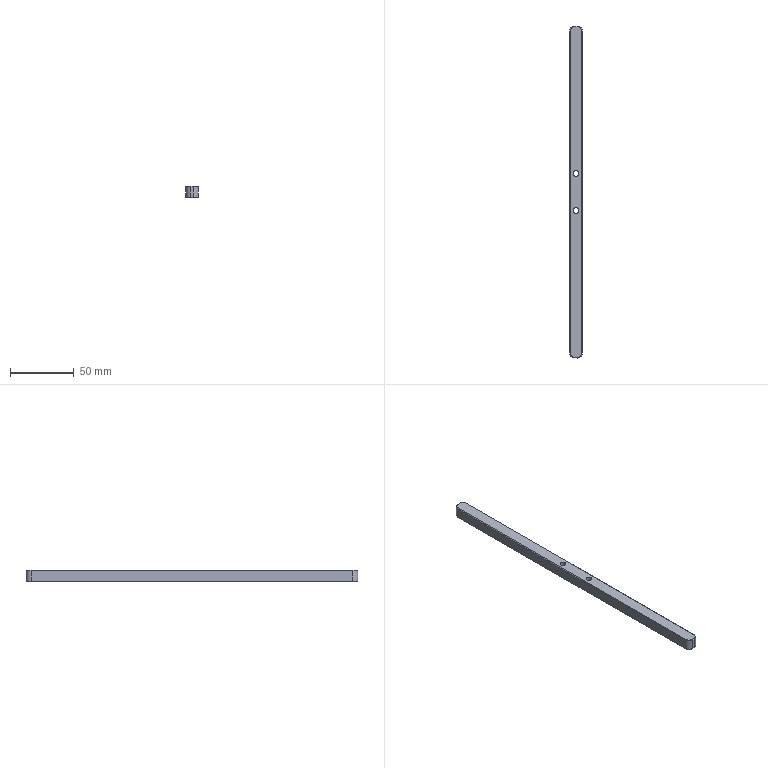Part | Creo | features DATUM PLANE 3, CHAMFER 1, COORDINATE SYSTEM 1, CURVE 1, PROTRUSION 1, ROUND 1 | 1 solid | 30 faces | box 10 x 259.76 x 9 mm | volume 22836 mm3 | plane 14 | cylinder 8 | cone 8 | commonest cylinder face diameters 4.5 x4 8 x4
STEP:
#1=CARTESIAN_POINT('',(0.,0.,0.));
#2=DIRECTION('',(0.,0.,1.));
#3=DIRECTION('',(1.,0.,0.));
#4=AXIS2_PLACEMENT_3D('',#1,#2,#3);
#5=CARTESIAN_POINT('',(-4.5,125.88,0.));
#6=VERTEX_POINT('',#5);
#7=CARTESIAN_POINT('',(-1.,129.38,0.));
#8=VERTEX_POINT('',#7);
#9=CARTESIAN_POINT('',(-1.,125.88,0.));
#10=DIRECTION('',(0.,0.,-1.));
#11=DIRECTION('',(-1.,0.,0.));
#12=AXIS2_PLACEMENT_3D('',#9,#10,#11);
#13=CIRCLE('',#12,3.5);
#14=EDGE_CURVE('',#6,#8,#13,.T.);
#15=ORIENTED_EDGE('',*,*,#14,.F.);
#16=CARTESIAN_POINT('',(-4.5,-125.88,0.));
#17=VERTEX_POINT('',#16);
#18=CARTESIAN_POINT('',(-4.5,-125.88,0.));
#19=DIRECTION('',(0.,1.,0.));
#20=VECTOR('',#19,251.76);
#21=LINE('',#18,#20);
#22=EDGE_CURVE('',#17,#6,#21,.T.);
#23=ORIENTED_EDGE('',*,*,#22,.F.);
#24=CARTESIAN_POINT('',(-1.,-129.38,-0.000000009));
#25=VERTEX_POINT('',#24);
#26=CARTESIAN_POINT('',(-1.,-125.88,0.));
#27=DIRECTION('',(0.,0.,-1.));
#28=DIRECTION('',(0.,-1.,0.));
#29=AXIS2_PLACEMENT_3D('',#26,#27,#28);
#30=CIRCLE('',#29,3.5);
#31=EDGE_CURVE('',#25,#17,#30,.T.);
#32=ORIENTED_EDGE('',*,*,#31,.F.);
#33=CARTESIAN_POINT('',(1.,-129.38,0.));
#34=VERTEX_POINT('',#33);
#35=CARTESIAN_POINT('',(1.,-129.38,0.));
#36=DIRECTION('',(-1.,0.000000005,-0.000000005));
#37=VECTOR('',#36,2.);
#38=LINE('',#35,#37);
#39=EDGE_CURVE('',#34,#25,#38,.T.);
#40=ORIENTED_EDGE('',*,*,#39,.F.);
#41=CARTESIAN_POINT('',(4.5,-125.88,-0.000000009));
#42=VERTEX_POINT('',#41);
#43=CARTESIAN_POINT('',(1.,-125.88,0.));
#44=DIRECTION('',(0.,0.,-1.));
#45=DIRECTION('',(1.,0.,0.));
#46=AXIS2_PLACEMENT_3D('',#43,#44,#45);
#47=CIRCLE('',#46,3.5);
#48=EDGE_CURVE('',#42,#34,#47,.T.);
#49=ORIENTED_EDGE('',*,*,#48,.F.);
#50=CARTESIAN_POINT('',(4.5,125.88,0.));
#51=VERTEX_POINT('',#50);
#52=CARTESIAN_POINT('',(4.5,125.88,0.));
#53=DIRECTION('',(0.,-1.,0.));
#54=VECTOR('',#53,251.76);
#55=LINE('',#52,#54);
#56=EDGE_CURVE('',#51,#42,#55,.T.);
#57=ORIENTED_EDGE('',*,*,#56,.F.);
#58=CARTESIAN_POINT('',(1.,129.38,-0.000000009));
#59=VERTEX_POINT('',#58);
#60=CARTESIAN_POINT('',(1.,125.88,0.));
#61=DIRECTION('',(0.,0.,-1.));
#62=DIRECTION('',(0.,1.,0.));
#63=AXIS2_PLACEMENT_3D('',#60,#61,#62);
#64=CIRCLE('',#63,3.5);
#65=EDGE_CURVE('',#59,#51,#64,.T.);
#66=ORIENTED_EDGE('',*,*,#65,.F.);
#67=CARTESIAN_POINT('',(-1.,129.38,0.));
#68=DIRECTION('',(1.,-0.000000005,-0.000000005));
#69=VECTOR('',#68,2.);
#70=LINE('',#67,#69);
#71=EDGE_CURVE('',#8,#59,#70,.T.);
#72=ORIENTED_EDGE('',*,*,#71,.F.);
#73=EDGE_LOOP('',(#15,#23,#32,#40,#49,#57,#66,#72));
#74=FACE_OUTER_BOUND('',#73,.F.);
#75=CARTESIAN_POINT('',(2.256,-14.5,0.));
#76=VERTEX_POINT('',#75);
#77=CARTESIAN_POINT('',(-2.244,-14.5,0.));
#78=VERTEX_POINT('',#77);
#79=CARTESIAN_POINT('',(0.006386,-14.5,0.));
#80=DIRECTION('',(0.,0.,-1.));
#81=DIRECTION('',(1.,0.,0.));
#82=AXIS2_PLACEMENT_3D('',#79,#80,#81);
#83=CIRCLE('',#82,2.25);
#84=EDGE_CURVE('',#76,#78,#83,.T.);
#85=ORIENTED_EDGE('',*,*,#84,.T.);
#86=CARTESIAN_POINT('',(0.006386,-14.5,0.));
#87=DIRECTION('',(0.,0.,-1.));
#88=DIRECTION('',(-1.,0.,0.));
#89=AXIS2_PLACEMENT_3D('',#86,#87,#88);
#90=CIRCLE('',#89,2.25);
#91=EDGE_CURVE('',#78,#76,#90,.T.);
#92=ORIENTED_EDGE('',*,*,#91,.T.);
#93=EDGE_LOOP('',(#85,#92));
#94=FACE_BOUND('',#93,.F.);
#95=CARTESIAN_POINT('',(2.256,14.5,0.));
#96=VERTEX_POINT('',#95);
#97=CARTESIAN_POINT('',(-2.244,14.5,0.));
#98=VERTEX_POINT('',#97);
#99=CARTESIAN_POINT('',(0.006386,14.5,0.));
#100=DIRECTION('',(0.,0.,-1.));
#101=DIRECTION('',(1.,0.,0.));
#102=AXIS2_PLACEMENT_3D('',#99,#100,#101);
#103=CIRCLE('',#102,2.25);
#104=EDGE_CURVE('',#96,#98,#103,.T.);
#105=ORIENTED_EDGE('',*,*,#104,.T.);
#106=CARTESIAN_POINT('',(0.006386,14.5,0.));
#107=DIRECTION('',(0.,0.,-1.));
#108=DIRECTION('',(-1.,0.,0.));
#109=AXIS2_PLACEMENT_3D('',#106,#107,#108);
#110=CIRCLE('',#109,2.25);
#111=EDGE_CURVE('',#98,#96,#110,.T.);
#112=ORIENTED_EDGE('',*,*,#111,.T.);
#113=EDGE_LOOP('',(#105,#112));
#114=FACE_BOUND('',#113,.F.);
#115=CARTESIAN_POINT('',(0.,0.,0.));
#116=DIRECTION('',(0.,0.,1.));
#117=DIRECTION('',(1.,0.,0.));
#118=AXIS2_PLACEMENT_3D('',#115,#116,#117);
#119=PLANE('',#118);
#120=ADVANCED_FACE('',(#74,#94,#114),#119,.F.);
#121=ORIENTED_EDGE('',*,*,#104,.F.);
#122=CARTESIAN_POINT('',(2.256,14.5,9.));
#123=VERTEX_POINT('',#122);
#124=CARTESIAN_POINT('',(2.256,14.5,0.));
#125=DIRECTION('',(0.,0.,1.));
#126=VECTOR('',#125,9.);
#127=LINE('',#124,#126);
#128=EDGE_CURVE('',#96,#123,#127,.T.);
#129=ORIENTED_EDGE('',*,*,#128,.T.);
#130=CARTESIAN_POINT('',(-2.244,14.5,9.));
#131=VERTEX_POINT('',#130);
#132=CARTESIAN_POINT('',(0.006386,14.5,9.));
#133=DIRECTION('',(0.,0.,-1.));
#134=DIRECTION('',(1.,0.,0.));
#135=AXIS2_PLACEMENT_3D('',#132,#133,#134);
#136=CIRCLE('',#135,2.25);
#137=EDGE_CURVE('',#123,#131,#136,.T.);
#138=ORIENTED_EDGE('',*,*,#137,.T.);
#139=CARTESIAN_POINT('',(-2.244,14.5,0.));
#140=DIRECTION('',(0.,0.,1.));
#141=VECTOR('',#140,9.);
#142=LINE('',#139,#141);
#143=EDGE_CURVE('',#98,#131,#142,.T.);
#144=ORIENTED_EDGE('',*,*,#143,.F.);
#145=EDGE_LOOP('',(#121,#129,#138,#144));
#146=FACE_OUTER_BOUND('',#145,.F.);
#147=CARTESIAN_POINT('',(0.006386,14.5,0.));
#148=DIRECTION('',(0.,0.,1.));
#149=DIRECTION('',(1.,0.,0.));
#150=AXIS2_PLACEMENT_3D('',#147,#148,#149);
#151=CYLINDRICAL_SURFACE('',#150,2.25);
#152=ADVANCED_FACE('',(#146),#151,.F.);
#153=ORIENTED_EDGE('',*,*,#111,.F.);
#154=ORIENTED_EDGE('',*,*,#143,.T.);
#155=CARTESIAN_POINT('',(0.006386,14.5,9.));
#156=DIRECTION('',(0.,0.,-1.));
#157=DIRECTION('',(-1.,0.,0.));
#158=AXIS2_PLACEMENT_3D('',#155,#156,#157);
#159=CIRCLE('',#158,2.25);
#160=EDGE_CURVE('',#131,#123,#159,.T.);
#161=ORIENTED_EDGE('',*,*,#160,.T.);
#162=ORIENTED_EDGE('',*,*,#128,.F.);
#163=EDGE_LOOP('',(#153,#154,#161,#162));
#164=FACE_OUTER_BOUND('',#163,.F.);
#165=CARTESIAN_POINT('',(0.006386,14.5,0.));
#166=DIRECTION('',(0.,0.,1.));
#167=DIRECTION('',(1.,0.,0.));
#168=AXIS2_PLACEMENT_3D('',#165,#166,#167);
#169=CYLINDRICAL_SURFACE('',#168,2.25);
#170=ADVANCED_FACE('',(#164),#169,.F.);
#171=CARTESIAN_POINT('',(-4.5,-125.88,9.));
#172=VERTEX_POINT('',#171);
#173=CARTESIAN_POINT('',(-1.,-129.38,9.));
#174=VERTEX_POINT('',#173);
#175=CARTESIAN_POINT('',(-1.,-125.88,9.));
#176=DIRECTION('',(0.,0.,1.));
#177=DIRECTION('',(-1.,0.,0.));
#178=AXIS2_PLACEMENT_3D('',#175,#176,#177);
#179=CIRCLE('',#178,3.5);
#180=EDGE_CURVE('',#172,#174,#179,.T.);
#181=ORIENTED_EDGE('',*,*,#180,.F.);
#182=CARTESIAN_POINT('',(-4.5,125.88,9.));
#183=VERTEX_POINT('',#182);
#184=CARTESIAN_POINT('',(-4.5,125.88,9.));
#185=DIRECTION('',(0.,-1.,0.));
#186=VECTOR('',#185,251.76);
#187=LINE('',#184,#186);
#188=EDGE_CURVE('',#183,#172,#187,.T.);
#189=ORIENTED_EDGE('',*,*,#188,.F.);
#190=CARTESIAN_POINT('',(-1.,129.38,9.));
#191=VERTEX_POINT('',#190);
#192=CARTESIAN_POINT('',(-1.,125.88,9.));
#193=DIRECTION('',(0.,0.,1.));
#194=DIRECTION('',(0.,1.,0.));
#195=AXIS2_PLACEMENT_3D('',#192,#193,#194);
#196=CIRCLE('',#195,3.5);
#197=EDGE_CURVE('',#191,#183,#196,.T.);
#198=ORIENTED_EDGE('',*,*,#197,.F.);
#199=CARTESIAN_POINT('',(1.,129.38,9.));
#200=VERTEX_POINT('',#199);
#201=CARTESIAN_POINT('',(1.,129.38,9.));
#202=DIRECTION('',(-1.,0.000000005,-0.000000005));
#203=VECTOR('',#202,2.);
#204=LINE('',#201,#203);
#205=EDGE_CURVE('',#200,#191,#204,.T.);
#206=ORIENTED_EDGE('',*,*,#205,.F.);
#207=CARTESIAN_POINT('',(4.5,125.88,9.));
#208=VERTEX_POINT('',#207);
#209=CARTESIAN_POINT('',(1.,125.88,9.));
#210=DIRECTION('',(0.,0.,1.));
#211=DIRECTION('',(1.,0.,0.));
#212=AXIS2_PLACEMENT_3D('',#209,#210,#211);
#213=CIRCLE('',#212,3.5);
#214=EDGE_CURVE('',#208,#200,#213,.T.);
#215=ORIENTED_EDGE('',*,*,#214,.F.);
#216=CARTESIAN_POINT('',(4.5,-125.88,9.));
#217=VERTEX_POINT('',#216);
#218=CARTESIAN_POINT('',(4.5,-125.88,9.));
#219=DIRECTION('',(0.,1.,0.));
#220=VECTOR('',#219,251.76);
#221=LINE('',#218,#220);
#222=EDGE_CURVE('',#217,#208,#221,.T.);
#223=ORIENTED_EDGE('',*,*,#222,.F.);
#224=CARTESIAN_POINT('',(1.,-129.38,9.));
#225=VERTEX_POINT('',#224);
#226=CARTESIAN_POINT('',(1.,-125.88,9.));
#227=DIRECTION('',(0.,0.,1.));
#228=DIRECTION('',(0.,-1.,0.));
#229=AXIS2_PLACEMENT_3D('',#226,#227,#228);
#230=CIRCLE('',#229,3.5);
#231=EDGE_CURVE('',#225,#217,#230,.T.);
#232=ORIENTED_EDGE('',*,*,#231,.F.);
#233=CARTESIAN_POINT('',(-1.,-129.38,9.));
#234=DIRECTION('',(1.,-0.000000005,-0.000000005));
#235=VECTOR('',#234,2.);
#236=LINE('',#233,#235);
#237=EDGE_CURVE('',#174,#225,#236,.T.);
#238=ORIENTED_EDGE('',*,*,#237,.F.);
#239=EDGE_LOOP('',(#181,#189,#198,#206,#215,#223,#232,#238));
#240=FACE_OUTER_BOUND('',#239,.F.);
#241=CARTESIAN_POINT('',(2.256,-14.5,9.));
#242=VERTEX_POINT('',#241);
#243=CARTESIAN_POINT('',(-2.244,-14.5,9.));
#244=VERTEX_POINT('',#243);
#245=CARTESIAN_POINT('',(0.006386,-14.5,9.));
#246=DIRECTION('',(0.,0.,-1.));
#247=DIRECTION('',(1.,0.,0.));
#248=AXIS2_PLACEMENT_3D('',#245,#246,#247);
#249=CIRCLE('',#248,2.25);
#250=EDGE_CURVE('',#242,#244,#249,.T.);
#251=ORIENTED_EDGE('',*,*,#250,.F.);
#252=CARTESIAN_POINT('',(0.006386,-14.5,9.));
#253=DIRECTION('',(0.,0.,-1.));
#254=DIRECTION('',(-1.,0.,0.));
#255=AXIS2_PLACEMENT_3D('',#252,#253,#254);
#256=CIRCLE('',#255,2.25);
#257=EDGE_CURVE('',#244,#242,#256,.T.);
#258=ORIENTED_EDGE('',*,*,#257,.F.);
#259=EDGE_LOOP('',(#251,#258));
#260=FACE_BOUND('',#259,.F.);
#261=ORIENTED_EDGE('',*,*,#137,.F.);
#262=ORIENTED_EDGE('',*,*,#160,.F.);
#263=EDGE_LOOP('',(#261,#262));
#264=FACE_BOUND('',#263,.F.);
#265=CARTESIAN_POINT('',(0.,0.,9.));
#266=DIRECTION('',(0.,0.,1.));
#267=DIRECTION('',(1.,0.,0.));
#268=AXIS2_PLACEMENT_3D('',#265,#266,#267);
#269=PLANE('',#268);
#270=ADVANCED_FACE('',(#240,#260,#264),#269,.T.);
#271=ORIENTED_EDGE('',*,*,#84,.F.);
#272=CARTESIAN_POINT('',(2.256,-14.5,0.));
#273=DIRECTION('',(0.,0.,1.));
#274=VECTOR('',#273,9.);
#275=LINE('',#272,#274);
#276=EDGE_CURVE('',#76,#242,#275,.T.);
#277=ORIENTED_EDGE('',*,*,#276,.T.);
#278=ORIENTED_EDGE('',*,*,#250,.T.);
#279=CARTESIAN_POINT('',(-2.244,-14.5,0.));
#280=DIRECTION('',(0.,0.,1.));
#281=VECTOR('',#280,9.);
#282=LINE('',#279,#281);
#283=EDGE_CURVE('',#78,#244,#282,.T.);
#284=ORIENTED_EDGE('',*,*,#283,.F.);
#285=EDGE_LOOP('',(#271,#277,#278,#284));
#286=FACE_OUTER_BOUND('',#285,.F.);
#287=CARTESIAN_POINT('',(0.006386,-14.5,0.));
#288=DIRECTION('',(0.,0.,1.));
#289=DIRECTION('',(1.,0.,0.));
#290=AXIS2_PLACEMENT_3D('',#287,#288,#289);
#291=CYLINDRICAL_SURFACE('',#290,2.25);
#292=ADVANCED_FACE('',(#286),#291,.F.);
#293=ORIENTED_EDGE('',*,*,#91,.F.);
#294=ORIENTED_EDGE('',*,*,#283,.T.);
#295=ORIENTED_EDGE('',*,*,#257,.T.);
#296=ORIENTED_EDGE('',*,*,#276,.F.);
#297=EDGE_LOOP('',(#293,#294,#295,#296));
#298=FACE_OUTER_BOUND('',#297,.F.);
#299=CARTESIAN_POINT('',(0.006386,-14.5,0.));
#300=DIRECTION('',(0.,0.,1.));
#301=DIRECTION('',(1.,0.,0.));
#302=AXIS2_PLACEMENT_3D('',#299,#300,#301);
#303=CYLINDRICAL_SURFACE('',#302,2.25);
#304=ADVANCED_FACE('',(#298),#303,.F.);
#305=ORIENTED_EDGE('',*,*,#180,.T.);
#306=CARTESIAN_POINT('',(-1.,-129.88,8.5));
#307=VERTEX_POINT('',#306);
#308=CARTESIAN_POINT('',(-1.,-129.38,9.));
#309=DIRECTION('',(0.000000006,-0.7071,-0.7071));
#310=VECTOR('',#309,0.7071);
#311=LINE('',#308,#310);
#312=EDGE_CURVE('',#174,#307,#311,.T.);
#313=ORIENTED_EDGE('',*,*,#312,.T.);
#314=CARTESIAN_POINT('',(-5.,-125.88,8.5));
#315=VERTEX_POINT('',#314);
#316=CARTESIAN_POINT('',(-1.,-125.88,8.5));
#317=DIRECTION('',(0.,0.,1.));
#318=DIRECTION('',(-1.,0.,0.));
#319=AXIS2_PLACEMENT_3D('',#316,#317,#318);
#320=CIRCLE('',#319,4.);
#321=EDGE_CURVE('',#315,#307,#320,.T.);
#322=ORIENTED_EDGE('',*,*,#321,.F.);
#323=CARTESIAN_POINT('',(-4.5,-125.88,9.));
#324=DIRECTION('',(-0.7071,0.,-0.7071));
#325=VECTOR('',#324,0.7071);
#326=LINE('',#323,#325);
#327=EDGE_CURVE('',#172,#315,#326,.T.);
#328=ORIENTED_EDGE('',*,*,#327,.F.);
#329=EDGE_LOOP('',(#305,#313,#322,#328));
#330=FACE_OUTER_BOUND('',#329,.F.);
#331=CARTESIAN_POINT('',(-1.,-125.88,8.75));
#332=DIRECTION('',(0.,0.,-1.));
#333=DIRECTION('',(0.,-1.,0.));
#334=AXIS2_PLACEMENT_3D('',#331,#332,#333);
#335=CONICAL_SURFACE('',#334,3.75,45.);
#336=ADVANCED_FACE('',(#330),#335,.T.);
#337=ORIENTED_EDGE('',*,*,#237,.T.);
#338=CARTESIAN_POINT('',(1.,-129.88,8.5));
#339=VERTEX_POINT('',#338);
#340=CARTESIAN_POINT('',(1.,-129.38,9.));
#341=DIRECTION('',(0.,-0.7071,-0.7071));
#342=VECTOR('',#341,0.7071);
#343=LINE('',#340,#342);
#344=EDGE_CURVE('',#225,#339,#343,.T.);
#345=ORIENTED_EDGE('',*,*,#344,.T.);
#346=CARTESIAN_POINT('',(-1.,-129.88,8.5));
#347=DIRECTION('',(1.,-0.000000004,-0.000000004));
#348=VECTOR('',#347,2.);
#349=LINE('',#346,#348);
#350=EDGE_CURVE('',#307,#339,#349,.T.);
#351=ORIENTED_EDGE('',*,*,#350,.F.);
#352=ORIENTED_EDGE('',*,*,#312,.F.);
#353=EDGE_LOOP('',(#337,#345,#351,#352));
#354=FACE_OUTER_BOUND('',#353,.F.);
#355=CARTESIAN_POINT('',(0.,-129.63,8.75));
#356=DIRECTION('',(0.,-0.7071,0.7071));
#357=DIRECTION('',(0.,-0.7071,-0.7071));
#358=AXIS2_PLACEMENT_3D('',#355,#356,#357);
#359=PLANE('',#358);
#360=ADVANCED_FACE('',(#354),#359,.T.);
#361=ORIENTED_EDGE('',*,*,#231,.T.);
#362=CARTESIAN_POINT('',(5.,-125.88,8.5));
#363=VERTEX_POINT('',#362);
#364=CARTESIAN_POINT('',(4.5,-125.88,9.));
#365=DIRECTION('',(0.7071,0.000000006,-0.7071));
#366=VECTOR('',#365,0.7071);
#367=LINE('',#364,#366);
#368=EDGE_CURVE('',#217,#363,#367,.T.);
#369=ORIENTED_EDGE('',*,*,#368,.T.);
#370=CARTESIAN_POINT('',(1.,-125.88,8.5));
#371=DIRECTION('',(0.,0.,1.));
#372=DIRECTION('',(0.,-1.,0.));
#373=AXIS2_PLACEMENT_3D('',#370,#371,#372);
#374=CIRCLE('',#373,4.);
#375=EDGE_CURVE('',#339,#363,#374,.T.);
#376=ORIENTED_EDGE('',*,*,#375,.F.);
#377=ORIENTED_EDGE('',*,*,#344,.F.);
#378=EDGE_LOOP('',(#361,#369,#376,#377));
#379=FACE_OUTER_BOUND('',#378,.F.);
#380=CARTESIAN_POINT('',(1.,-125.88,8.75));
#381=DIRECTION('',(0.,0.,-1.));
#382=DIRECTION('',(0.,-1.,0.));
#383=AXIS2_PLACEMENT_3D('',#380,#381,#382);
#384=CONICAL_SURFACE('',#383,3.75,45.);
#385=ADVANCED_FACE('',(#379),#384,.T.);
#386=ORIENTED_EDGE('',*,*,#222,.T.);
#387=CARTESIAN_POINT('',(5.,125.88,8.5));
#388=VERTEX_POINT('',#387);
#389=CARTESIAN_POINT('',(4.5,125.88,9.));
#390=DIRECTION('',(0.7071,0.,-0.7071));
#391=VECTOR('',#390,0.7071);
#392=LINE('',#389,#391);
#393=EDGE_CURVE('',#208,#388,#392,.T.);
#394=ORIENTED_EDGE('',*,*,#393,.T.);
#395=CARTESIAN_POINT('',(5.,-125.88,8.5));
#396=DIRECTION('',(0.,1.,0.));
#397=VECTOR('',#396,251.76);
#398=LINE('',#395,#397);
#399=EDGE_CURVE('',#363,#388,#398,.T.);
#400=ORIENTED_EDGE('',*,*,#399,.F.);
#401=ORIENTED_EDGE('',*,*,#368,.F.);
#402=EDGE_LOOP('',(#386,#394,#400,#401));
#403=FACE_OUTER_BOUND('',#402,.F.);
#404=CARTESIAN_POINT('',(4.75,0.,8.75));
#405=DIRECTION('',(0.7071,0.,0.7071));
#406=DIRECTION('',(0.7071,0.,-0.7071));
#407=AXIS2_PLACEMENT_3D('',#404,#405,#406);
#408=PLANE('',#407);
#409=ADVANCED_FACE('',(#403),#408,.T.);
#410=ORIENTED_EDGE('',*,*,#214,.T.);
#411=CARTESIAN_POINT('',(1.,129.88,8.5));
#412=VERTEX_POINT('',#411);
#413=CARTESIAN_POINT('',(1.,129.38,9.));
#414=DIRECTION('',(-0.000000006,0.7071,-0.7071));
#415=VECTOR('',#414,0.7071);
#416=LINE('',#413,#415);
#417=EDGE_CURVE('',#200,#412,#416,.T.);
#418=ORIENTED_EDGE('',*,*,#417,.T.);
#419=CARTESIAN_POINT('',(1.,125.88,8.5));
#420=DIRECTION('',(0.,0.,1.));
#421=DIRECTION('',(1.,0.,0.));
#422=AXIS2_PLACEMENT_3D('',#419,#420,#421);
#423=CIRCLE('',#422,4.);
#424=EDGE_CURVE('',#388,#412,#423,.T.);
#425=ORIENTED_EDGE('',*,*,#424,.F.);
#426=ORIENTED_EDGE('',*,*,#393,.F.);
#427=EDGE_LOOP('',(#410,#418,#425,#426));
#428=FACE_OUTER_BOUND('',#427,.F.);
#429=CARTESIAN_POINT('',(1.,125.88,8.75));
#430=DIRECTION('',(0.,0.,-1.));
#431=DIRECTION('',(0.,-1.,0.));
#432=AXIS2_PLACEMENT_3D('',#429,#430,#431);
#433=CONICAL_SURFACE('',#432,3.75,45.);
#434=ADVANCED_FACE('',(#428),#433,.T.);
#435=ORIENTED_EDGE('',*,*,#205,.T.);
#436=CARTESIAN_POINT('',(-1.,129.88,8.5));
#437=VERTEX_POINT('',#436);
#438=CARTESIAN_POINT('',(-1.,129.38,9.));
#439=DIRECTION('',(0.,0.7071,-0.7071));
#440=VECTOR('',#439,0.7071);
#441=LINE('',#438,#440);
#442=EDGE_CURVE('',#191,#437,#441,.T.);
#443=ORIENTED_EDGE('',*,*,#442,.T.);
#444=CARTESIAN_POINT('',(1.,129.88,8.5));
#445=DIRECTION('',(-1.,0.000000004,-0.000000004));
#446=VECTOR('',#445,2.);
#447=LINE('',#444,#446);
#448=EDGE_CURVE('',#412,#437,#447,.T.);
#449=ORIENTED_EDGE('',*,*,#448,.F.);
#450=ORIENTED_EDGE('',*,*,#417,.F.);
#451=EDGE_LOOP('',(#435,#443,#449,#450));
#452=FACE_OUTER_BOUND('',#451,.F.);
#453=CARTESIAN_POINT('',(0.,129.63,8.75));
#454=DIRECTION('',(0.,0.7071,0.7071));
#455=DIRECTION('',(0.,0.7071,-0.7071));
#456=AXIS2_PLACEMENT_3D('',#453,#454,#455);
#457=PLANE('',#456);
#458=ADVANCED_FACE('',(#452),#457,.T.);
#459=ORIENTED_EDGE('',*,*,#197,.T.);
#460=CARTESIAN_POINT('',(-5.,125.88,8.5));
#461=VERTEX_POINT('',#460);
#462=CARTESIAN_POINT('',(-4.5,125.88,9.));
#463=DIRECTION('',(-0.7071,-0.000000006,-0.7071));
#464=VECTOR('',#463,0.7071);
#465=LINE('',#462,#464);
#466=EDGE_CURVE('',#183,#461,#465,.T.);
#467=ORIENTED_EDGE('',*,*,#466,.T.);
#468=CARTESIAN_POINT('',(-1.,125.88,8.5));
#469=DIRECTION('',(0.,0.,1.));
#470=DIRECTION('',(0.,1.,0.));
#471=AXIS2_PLACEMENT_3D('',#468,#469,#470);
#472=CIRCLE('',#471,4.);
#473=EDGE_CURVE('',#437,#461,#472,.T.);
#474=ORIENTED_EDGE('',*,*,#473,.F.);
#475=ORIENTED_EDGE('',*,*,#442,.F.);
#476=EDGE_LOOP('',(#459,#467,#474,#475));
#477=FACE_OUTER_BOUND('',#476,.F.);
#478=CARTESIAN_POINT('',(-1.,125.88,8.75));
#479=DIRECTION('',(0.,0.,-1.));
#480=DIRECTION('',(0.,-1.,0.));
#481=AXIS2_PLACEMENT_3D('',#478,#479,#480);
#482=CONICAL_SURFACE('',#481,3.75,45.);
#483=ADVANCED_FACE('',(#477),#482,.T.);
#484=ORIENTED_EDGE('',*,*,#188,.T.);
#485=ORIENTED_EDGE('',*,*,#327,.T.);
#486=CARTESIAN_POINT('',(-5.,125.88,8.5));
#487=DIRECTION('',(0.,-1.,0.));
#488=VECTOR('',#487,251.76);
#489=LINE('',#486,#488);
#490=EDGE_CURVE('',#461,#315,#489,.T.);
#491=ORIENTED_EDGE('',*,*,#490,.F.);
#492=ORIENTED_EDGE('',*,*,#466,.F.);
#493=EDGE_LOOP('',(#484,#485,#491,#492));
#494=FACE_OUTER_BOUND('',#493,.F.);
#495=CARTESIAN_POINT('',(-4.75,0.,8.75));
#496=DIRECTION('',(-0.7071,0.,0.7071));
#497=DIRECTION('',(-0.7071,0.,-0.7071));
#498=AXIS2_PLACEMENT_3D('',#495,#496,#497);
#499=PLANE('',#498);
#500=ADVANCED_FACE('',(#494),#499,.T.);
#501=ORIENTED_EDGE('',*,*,#490,.T.);
#502=CARTESIAN_POINT('',(-5.,-125.88,0.5));
#503=VERTEX_POINT('',#502);
#504=CARTESIAN_POINT('',(-5.,-125.88,8.5));
#505=DIRECTION('',(0.,0.,-1.));
#506=VECTOR('',#505,8.);
#507=LINE('',#504,#506);
#508=EDGE_CURVE('',#315,#503,#507,.T.);
#509=ORIENTED_EDGE('',*,*,#508,.T.);
#510=CARTESIAN_POINT('',(-5.,125.88,0.5));
#511=VERTEX_POINT('',#510);
#512=CARTESIAN_POINT('',(-5.,-125.88,0.5));
#513=DIRECTION('',(0.,1.,0.));
#514=VECTOR('',#513,251.76);
#515=LINE('',#512,#514);
#516=EDGE_CURVE('',#503,#511,#515,.T.);
#517=ORIENTED_EDGE('',*,*,#516,.T.);
#518=CARTESIAN_POINT('',(-5.,125.88,8.5));
#519=DIRECTION('',(0.,0.,-1.));
#520=VECTOR('',#519,8.);
#521=LINE('',#518,#520);
#522=EDGE_CURVE('',#461,#511,#521,.T.);
#523=ORIENTED_EDGE('',*,*,#522,.F.);
#524=EDGE_LOOP('',(#501,#509,#517,#523));
#525=FACE_OUTER_BOUND('',#524,.F.);
#526=CARTESIAN_POINT('',(-5.,129.88,0.));
#527=DIRECTION('',(-1.,0.,0.));
#528=DIRECTION('',(0.,-1.,0.));
#529=AXIS2_PLACEMENT_3D('',#526,#527,#528);
#530=PLANE('',#529);
#531=ADVANCED_FACE('',(#525),#530,.T.);
#532=ORIENTED_EDGE('',*,*,#321,.T.);
#533=CARTESIAN_POINT('',(-1.,-129.88,0.5));
#534=VERTEX_POINT('',#533);
#535=CARTESIAN_POINT('',(-1.,-129.88,8.5));
#536=DIRECTION('',(0.,0.,-1.));
#537=VECTOR('',#536,8.);
#538=LINE('',#535,#537);
#539=EDGE_CURVE('',#307,#534,#538,.T.);
#540=ORIENTED_EDGE('',*,*,#539,.T.);
#541=CARTESIAN_POINT('',(-1.,-125.88,0.5));
#542=DIRECTION('',(0.,0.,-1.));
#543=DIRECTION('',(0.,-1.,0.));
#544=AXIS2_PLACEMENT_3D('',#541,#542,#543);
#545=CIRCLE('',#544,4.);
#546=EDGE_CURVE('',#534,#503,#545,.T.);
#547=ORIENTED_EDGE('',*,*,#546,.T.);
#548=ORIENTED_EDGE('',*,*,#508,.F.);
#549=EDGE_LOOP('',(#532,#540,#547,#548));
#550=FACE_OUTER_BOUND('',#549,.F.);
#551=CARTESIAN_POINT('',(-1.,-125.88,20.732));
#552=DIRECTION('',(0.,0.,-1.));
#553=DIRECTION('',(0.,-1.,0.));
#554=AXIS2_PLACEMENT_3D('',#551,#552,#553);
#555=CYLINDRICAL_SURFACE('',#554,4.);
#556=ADVANCED_FACE('',(#550),#555,.T.);
#557=ORIENTED_EDGE('',*,*,#350,.T.);
#558=CARTESIAN_POINT('',(1.,-129.88,0.5));
#559=VERTEX_POINT('',#558);
#560=CARTESIAN_POINT('',(1.,-129.88,8.5));
#561=DIRECTION('',(0.,0.,-1.));
#562=VECTOR('',#561,8.);
#563=LINE('',#560,#562);
#564=EDGE_CURVE('',#339,#559,#563,.T.);
#565=ORIENTED_EDGE('',*,*,#564,.T.);
#566=CARTESIAN_POINT('',(1.,-129.88,0.5));
#567=DIRECTION('',(-1.,0.000000004,-0.000000004));
#568=VECTOR('',#567,2.);
#569=LINE('',#566,#568);
#570=EDGE_CURVE('',#559,#534,#569,.T.);
#571=ORIENTED_EDGE('',*,*,#570,.T.);
#572=ORIENTED_EDGE('',*,*,#539,.F.);
#573=EDGE_LOOP('',(#557,#565,#571,#572));
#574=FACE_OUTER_BOUND('',#573,.F.);
#575=CARTESIAN_POINT('',(-5.,-129.88,0.));
#576=DIRECTION('',(0.,-1.,0.));
#577=DIRECTION('',(1.,0.,0.));
#578=AXIS2_PLACEMENT_3D('',#575,#576,#577);
#579=PLANE('',#578);
#580=ADVANCED_FACE('',(#574),#579,.T.);
#581=ORIENTED_EDGE('',*,*,#375,.T.);
#582=CARTESIAN_POINT('',(5.,-125.88,0.5));
#583=VERTEX_POINT('',#582);
#584=CARTESIAN_POINT('',(5.,-125.88,8.5));
#585=DIRECTION('',(0.,0.,-1.));
#586=VECTOR('',#585,8.);
#587=LINE('',#584,#586);
#588=EDGE_CURVE('',#363,#583,#587,.T.);
#589=ORIENTED_EDGE('',*,*,#588,.T.);
#590=CARTESIAN_POINT('',(1.,-125.88,0.5));
#591=DIRECTION('',(0.,0.,-1.));
#592=DIRECTION('',(1.,0.,0.));
#593=AXIS2_PLACEMENT_3D('',#590,#591,#592);
#594=CIRCLE('',#593,4.);
#595=EDGE_CURVE('',#583,#559,#594,.T.);
#596=ORIENTED_EDGE('',*,*,#595,.T.);
#597=ORIENTED_EDGE('',*,*,#564,.F.);
#598=EDGE_LOOP('',(#581,#589,#596,#597));
#599=FACE_OUTER_BOUND('',#598,.F.);
#600=CARTESIAN_POINT('',(1.,-125.88,20.732));
#601=DIRECTION('',(0.,0.,-1.));
#602=DIRECTION('',(1.,0.,0.));
#603=AXIS2_PLACEMENT_3D('',#600,#601,#602);
#604=CYLINDRICAL_SURFACE('',#603,4.);
#605=ADVANCED_FACE('',(#599),#604,.T.);
#606=ORIENTED_EDGE('',*,*,#399,.T.);
#607=CARTESIAN_POINT('',(5.,125.88,0.5));
#608=VERTEX_POINT('',#607);
#609=CARTESIAN_POINT('',(5.,125.88,8.5));
#610=DIRECTION('',(0.,0.,-1.));
#611=VECTOR('',#610,8.);
#612=LINE('',#609,#611);
#613=EDGE_CURVE('',#388,#608,#612,.T.);
#614=ORIENTED_EDGE('',*,*,#613,.T.);
#615=CARTESIAN_POINT('',(5.,125.88,0.5));
#616=DIRECTION('',(0.,-1.,0.));
#617=VECTOR('',#616,251.76);
#618=LINE('',#615,#617);
#619=EDGE_CURVE('',#608,#583,#618,.T.);
#620=ORIENTED_EDGE('',*,*,#619,.T.);
#621=ORIENTED_EDGE('',*,*,#588,.F.);
#622=EDGE_LOOP('',(#606,#614,#620,#621));
#623=FACE_OUTER_BOUND('',#622,.F.);
#624=CARTESIAN_POINT('',(5.,-129.88,0.));
#625=DIRECTION('',(1.,0.,0.));
#626=DIRECTION('',(0.,1.,0.));
#627=AXIS2_PLACEMENT_3D('',#624,#625,#626);
#628=PLANE('',#627);
#629=ADVANCED_FACE('',(#623),#628,.T.);
#630=ORIENTED_EDGE('',*,*,#424,.T.);
#631=CARTESIAN_POINT('',(1.,129.88,0.5));
#632=VERTEX_POINT('',#631);
#633=CARTESIAN_POINT('',(1.,129.88,8.5));
#634=DIRECTION('',(0.,0.,-1.));
#635=VECTOR('',#634,8.);
#636=LINE('',#633,#635);
#637=EDGE_CURVE('',#412,#632,#636,.T.);
#638=ORIENTED_EDGE('',*,*,#637,.T.);
#639=CARTESIAN_POINT('',(1.,125.88,0.5));
#640=DIRECTION('',(0.,0.,-1.));
#641=DIRECTION('',(0.,1.,0.));
#642=AXIS2_PLACEMENT_3D('',#639,#640,#641);
#643=CIRCLE('',#642,4.);
#644=EDGE_CURVE('',#632,#608,#643,.T.);
#645=ORIENTED_EDGE('',*,*,#644,.T.);
#646=ORIENTED_EDGE('',*,*,#613,.F.);
#647=EDGE_LOOP('',(#630,#638,#645,#646));
#648=FACE_OUTER_BOUND('',#647,.F.);
#649=CARTESIAN_POINT('',(1.,125.88,20.732));
#650=DIRECTION('',(0.,0.,-1.));
#651=DIRECTION('',(0.,1.,0.));
#652=AXIS2_PLACEMENT_3D('',#649,#650,#651);
#653=CYLINDRICAL_SURFACE('',#652,4.);
#654=ADVANCED_FACE('',(#648),#653,.T.);
#655=ORIENTED_EDGE('',*,*,#448,.T.);
#656=CARTESIAN_POINT('',(-1.,129.88,0.5));
#657=VERTEX_POINT('',#656);
#658=CARTESIAN_POINT('',(-1.,129.88,8.5));
#659=DIRECTION('',(0.,0.,-1.));
#660=VECTOR('',#659,8.);
#661=LINE('',#658,#660);
#662=EDGE_CURVE('',#437,#657,#661,.T.);
#663=ORIENTED_EDGE('',*,*,#662,.T.);
#664=CARTESIAN_POINT('',(-1.,129.88,0.5));
#665=DIRECTION('',(1.,-0.000000004,-0.000000004));
#666=VECTOR('',#665,2.);
#667=LINE('',#664,#666);
#668=EDGE_CURVE('',#657,#632,#667,.T.);
#669=ORIENTED_EDGE('',*,*,#668,.T.);
#670=ORIENTED_EDGE('',*,*,#637,.F.);
#671=EDGE_LOOP('',(#655,#663,#669,#670));
#672=FACE_OUTER_BOUND('',#671,.F.);
#673=CARTESIAN_POINT('',(5.,129.88,0.));
#674=DIRECTION('',(0.,1.,0.));
#675=DIRECTION('',(-1.,0.,0.));
#676=AXIS2_PLACEMENT_3D('',#673,#674,#675);
#677=PLANE('',#676);
#678=ADVANCED_FACE('',(#672),#677,.T.);
#679=ORIENTED_EDGE('',*,*,#473,.T.);
#680=ORIENTED_EDGE('',*,*,#522,.T.);
#681=CARTESIAN_POINT('',(-1.,125.88,0.5));
#682=DIRECTION('',(0.,0.,-1.));
#683=DIRECTION('',(-1.,0.,0.));
#684=AXIS2_PLACEMENT_3D('',#681,#682,#683);
#685=CIRCLE('',#684,4.);
#686=EDGE_CURVE('',#511,#657,#685,.T.);
#687=ORIENTED_EDGE('',*,*,#686,.T.);
#688=ORIENTED_EDGE('',*,*,#662,.F.);
#689=EDGE_LOOP('',(#679,#680,#687,#688));
#690=FACE_OUTER_BOUND('',#689,.F.);
#691=CARTESIAN_POINT('',(-1.,125.88,20.732));
#692=DIRECTION('',(0.,0.,-1.));
#693=DIRECTION('',(-1.,0.,0.));
#694=AXIS2_PLACEMENT_3D('',#691,#692,#693);
#695=CYLINDRICAL_SURFACE('',#694,4.);
#696=ADVANCED_FACE('',(#690),#695,.T.);
#697=ORIENTED_EDGE('',*,*,#14,.T.);
#698=CARTESIAN_POINT('',(-1.,129.38,0.));
#699=DIRECTION('',(0.,0.7071,0.7071));
#700=VECTOR('',#699,0.7071);
#701=LINE('',#698,#700);
#702=EDGE_CURVE('',#8,#657,#701,.T.);
#703=ORIENTED_EDGE('',*,*,#702,.T.);
#704=ORIENTED_EDGE('',*,*,#686,.F.);
#705=CARTESIAN_POINT('',(-4.5,125.88,-0.000000009));
#706=DIRECTION('',(-0.7071,-0.000000006,0.7071));
#707=VECTOR('',#706,0.7071);
#708=LINE('',#705,#707);
#709=EDGE_CURVE('',#6,#511,#708,.T.);
#710=ORIENTED_EDGE('',*,*,#709,.F.);
#711=EDGE_LOOP('',(#697,#703,#704,#710));
#712=FACE_OUTER_BOUND('',#711,.F.);
#713=CARTESIAN_POINT('',(-1.,125.88,0.25));
#714=DIRECTION('',(0.,0.,1.));
#715=DIRECTION('',(0.,-1.,0.));
#716=AXIS2_PLACEMENT_3D('',#713,#714,#715);
#717=CONICAL_SURFACE('',#716,3.75,45.);
#718=ADVANCED_FACE('',(#712),#717,.T.);
#719=ORIENTED_EDGE('',*,*,#71,.T.);
#720=CARTESIAN_POINT('',(1.,129.38,-0.000000009));
#721=DIRECTION('',(-0.000000006,0.7071,0.7071));
#722=VECTOR('',#721,0.7071);
#723=LINE('',#720,#722);
#724=EDGE_CURVE('',#59,#632,#723,.T.);
#725=ORIENTED_EDGE('',*,*,#724,.T.);
#726=ORIENTED_EDGE('',*,*,#668,.F.);
#727=ORIENTED_EDGE('',*,*,#702,.F.);
#728=EDGE_LOOP('',(#719,#725,#726,#727));
#729=FACE_OUTER_BOUND('',#728,.F.);
#730=CARTESIAN_POINT('',(0.,129.63,0.25));
#731=DIRECTION('',(0.,0.7071,-0.7071));
#732=DIRECTION('',(0.,0.7071,0.7071));
#733=AXIS2_PLACEMENT_3D('',#730,#731,#732);
#734=PLANE('',#733);
#735=ADVANCED_FACE('',(#729),#734,.T.);
#736=ORIENTED_EDGE('',*,*,#65,.T.);
#737=CARTESIAN_POINT('',(4.5,125.88,0.));
#738=DIRECTION('',(0.7071,0.,0.7071));
#739=VECTOR('',#738,0.7071);
#740=LINE('',#737,#739);
#741=EDGE_CURVE('',#51,#608,#740,.T.);
#742=ORIENTED_EDGE('',*,*,#741,.T.);
#743=ORIENTED_EDGE('',*,*,#644,.F.);
#744=ORIENTED_EDGE('',*,*,#724,.F.);
#745=EDGE_LOOP('',(#736,#742,#743,#744));
#746=FACE_OUTER_BOUND('',#745,.F.);
#747=CARTESIAN_POINT('',(1.,125.88,0.25));
#748=DIRECTION('',(0.,0.,1.));
#749=DIRECTION('',(0.,-1.,0.));
#750=AXIS2_PLACEMENT_3D('',#747,#748,#749);
#751=CONICAL_SURFACE('',#750,3.75,45.);
#752=ADVANCED_FACE('',(#746),#751,.T.);
#753=ORIENTED_EDGE('',*,*,#56,.T.);
#754=CARTESIAN_POINT('',(4.5,-125.88,-0.000000009));
#755=DIRECTION('',(0.7071,0.000000006,0.7071));
#756=VECTOR('',#755,0.7071);
#757=LINE('',#754,#756);
#758=EDGE_CURVE('',#42,#583,#757,.T.);
#759=ORIENTED_EDGE('',*,*,#758,.T.);
#760=ORIENTED_EDGE('',*,*,#619,.F.);
#761=ORIENTED_EDGE('',*,*,#741,.F.);
#762=EDGE_LOOP('',(#753,#759,#760,#761));
#763=FACE_OUTER_BOUND('',#762,.F.);
#764=CARTESIAN_POINT('',(4.75,0.,0.25));
#765=DIRECTION('',(0.7071,0.,-0.7071));
#766=DIRECTION('',(0.7071,0.,0.7071));
#767=AXIS2_PLACEMENT_3D('',#764,#765,#766);
#768=PLANE('',#767);
#769=ADVANCED_FACE('',(#763),#768,.T.);
#770=ORIENTED_EDGE('',*,*,#48,.T.);
#771=CARTESIAN_POINT('',(1.,-129.38,0.));
#772=DIRECTION('',(0.,-0.7071,0.7071));
#773=VECTOR('',#772,0.7071);
#774=LINE('',#771,#773);
#775=EDGE_CURVE('',#34,#559,#774,.T.);
#776=ORIENTED_EDGE('',*,*,#775,.T.);
#777=ORIENTED_EDGE('',*,*,#595,.F.);
#778=ORIENTED_EDGE('',*,*,#758,.F.);
#779=EDGE_LOOP('',(#770,#776,#777,#778));
#780=FACE_OUTER_BOUND('',#779,.F.);
#781=CARTESIAN_POINT('',(1.,-125.88,0.25));
#782=DIRECTION('',(0.,0.,1.));
#783=DIRECTION('',(0.,-1.,0.));
#784=AXIS2_PLACEMENT_3D('',#781,#782,#783);
#785=CONICAL_SURFACE('',#784,3.75,45.);
#786=ADVANCED_FACE('',(#780),#785,.T.);
#787=ORIENTED_EDGE('',*,*,#39,.T.);
#788=CARTESIAN_POINT('',(-1.,-129.38,-0.000000009));
#789=DIRECTION('',(0.000000006,-0.7071,0.7071));
#790=VECTOR('',#789,0.7071);
#791=LINE('',#788,#790);
#792=EDGE_CURVE('',#25,#534,#791,.T.);
#793=ORIENTED_EDGE('',*,*,#792,.T.);
#794=ORIENTED_EDGE('',*,*,#570,.F.);
#795=ORIENTED_EDGE('',*,*,#775,.F.);
#796=EDGE_LOOP('',(#787,#793,#794,#795));
#797=FACE_OUTER_BOUND('',#796,.F.);
#798=CARTESIAN_POINT('',(0.,-129.63,0.25));
#799=DIRECTION('',(0.,-0.7071,-0.7071));
#800=DIRECTION('',(0.,-0.7071,0.7071));
#801=AXIS2_PLACEMENT_3D('',#798,#799,#800);
#802=PLANE('',#801);
#803=ADVANCED_FACE('',(#797),#802,.T.);
#804=ORIENTED_EDGE('',*,*,#31,.T.);
#805=CARTESIAN_POINT('',(-4.5,-125.88,0.));
#806=DIRECTION('',(-0.7071,0.,0.7071));
#807=VECTOR('',#806,0.7071);
#808=LINE('',#805,#807);
#809=EDGE_CURVE('',#17,#503,#808,.T.);
#810=ORIENTED_EDGE('',*,*,#809,.T.);
#811=ORIENTED_EDGE('',*,*,#546,.F.);
#812=ORIENTED_EDGE('',*,*,#792,.F.);
#813=EDGE_LOOP('',(#804,#810,#811,#812));
#814=FACE_OUTER_BOUND('',#813,.F.);
#815=CARTESIAN_POINT('',(-1.,-125.88,0.25));
#816=DIRECTION('',(0.,0.,1.));
#817=DIRECTION('',(0.,-1.,0.));
#818=AXIS2_PLACEMENT_3D('',#815,#816,#817);
#819=CONICAL_SURFACE('',#818,3.75,45.);
#820=ADVANCED_FACE('',(#814),#819,.T.);
#821=ORIENTED_EDGE('',*,*,#22,.T.);
#822=ORIENTED_EDGE('',*,*,#709,.T.);
#823=ORIENTED_EDGE('',*,*,#516,.F.);
#824=ORIENTED_EDGE('',*,*,#809,.F.);
#825=EDGE_LOOP('',(#821,#822,#823,#824));
#826=FACE_OUTER_BOUND('',#825,.F.);
#827=CARTESIAN_POINT('',(-4.75,0.,0.25));
#828=DIRECTION('',(-0.7071,0.,-0.7071));
#829=DIRECTION('',(-0.7071,0.,0.7071));
#830=AXIS2_PLACEMENT_3D('',#827,#828,#829);
#831=PLANE('',#830);
#832=ADVANCED_FACE('',(#826),#831,.T.);
#833=CLOSED_SHELL('',(#120,#152,#170,#270,#292,#304,#336,#360,#385,#409,#434,#458,#483,#500,#531,#556,#580,#605,#629,#654,#678,#696,#718,#735,#752,#769,#786,#803,#820,#832));
#834=MANIFOLD_SOLID_BREP('',#833);
#835=(LENGTH_UNIT()NAMED_UNIT(*)SI_UNIT(.MILLI.,.METRE.));
#836=UNCERTAINTY_MEASURE_WITH_UNIT(LENGTH_MEASURE(0.02601),#835,'','');
#837=(NAMED_UNIT(*)PLANE_ANGLE_UNIT()SI_UNIT($,.RADIAN.));
#838=PLANE_ANGLE_MEASURE_WITH_UNIT(PLANE_ANGLE_MEASURE(0.01745),#837);
#839=(CONVERSION_BASED_UNIT('DEGREE',#838)NAMED_UNIT(*)PLANE_ANGLE_UNIT());
#840=(NAMED_UNIT(*)SI_UNIT($,.STERADIAN.)SOLID_ANGLE_UNIT());
#841=(GEOMETRIC_REPRESENTATION_CONTEXT(3)GLOBAL_UNCERTAINTY_ASSIGNED_CONTEXT((#836))GLOBAL_UNIT_ASSIGNED_CONTEXT((#835,#839,#840))REPRESENTATION_CONTEXT('',''));
#842=ADVANCED_BREP_SHAPE_REPRESENTATION('',(#4,#834),#841);